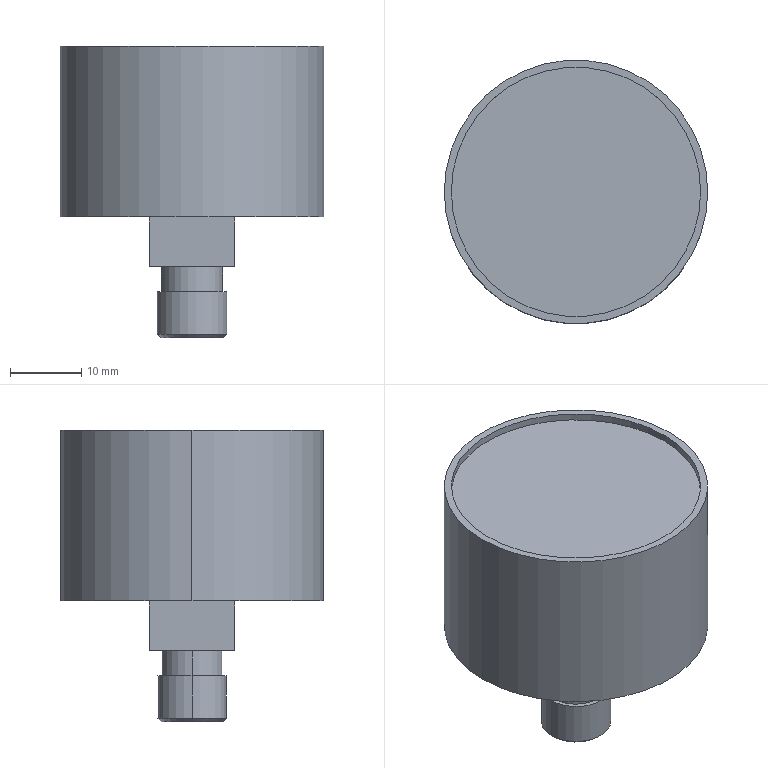Part | NX | 1 solid | 20 faces | box 37 x 37 x 41 mm | volume 26532 mm3 | plane 10 | cylinder 8 | cone 2 | commonest cylinder face diameters 8.57 x2 9.73 x2 35 x2 37 x2
STEP:
#1=CARTESIAN_POINT('',(18.5,0.,0.));
#2=VERTEX_POINT('',#1);
#3=CARTESIAN_POINT('',(-18.5,0.,0.));
#4=VERTEX_POINT('',#3);
#5=CARTESIAN_POINT('',(0.,0.,0.));
#6=DIRECTION('',(0.,0.,-1.));
#7=DIRECTION('',(1.,0.,0.));
#8=AXIS2_PLACEMENT_3D('',#5,#6,#7);
#9=CIRCLE('',#8,18.5);
#10=EDGE_CURVE('',#2,#4,#9,.T.);
#11=ORIENTED_EDGE('',*,*,#10,.T.);
#12=CARTESIAN_POINT('',(-18.5,0.,-24.));
#13=VERTEX_POINT('',#12);
#14=CARTESIAN_POINT('',(-18.5,0.,0.));
#15=DIRECTION('',(0.,0.,1.));
#16=VECTOR('',#15,1000.);
#17=LINE('',#14,#16);
#18=EDGE_CURVE('',#4,#13,#17,.F.);
#19=ORIENTED_EDGE('',*,*,#18,.T.);
#20=CARTESIAN_POINT('',(18.5,0.,-24.));
#21=VERTEX_POINT('',#20);
#22=CARTESIAN_POINT('',(0.,0.,-24.));
#23=DIRECTION('',(0.,0.,1.));
#24=DIRECTION('',(1.,0.,0.));
#25=AXIS2_PLACEMENT_3D('',#22,#23,#24);
#26=CIRCLE('',#25,18.5);
#27=EDGE_CURVE('',#13,#21,#26,.T.);
#28=ORIENTED_EDGE('',*,*,#27,.T.);
#29=CARTESIAN_POINT('',(18.5,0.,0.));
#30=DIRECTION('',(0.,0.,1.));
#31=VECTOR('',#30,1000.);
#32=LINE('',#29,#31);
#33=EDGE_CURVE('',#2,#21,#32,.F.);
#34=ORIENTED_EDGE('',*,*,#33,.F.);
#35=EDGE_LOOP('',(#11,#19,#28,#34));
#36=FACE_BOUND('',#35,.T.);
#37=CARTESIAN_POINT('',(0.,0.,0.));
#38=DIRECTION('',(0.,0.,1.));
#39=DIRECTION('',(1.,0.,0.));
#40=AXIS2_PLACEMENT_3D('',#37,#38,#39);
#41=CYLINDRICAL_SURFACE('',#40,18.5);
#42=ADVANCED_FACE('',(#36),#41,.T.);
#43=CARTESIAN_POINT('',(-4.285,0.,-41.));
#44=VERTEX_POINT('',#43);
#45=CARTESIAN_POINT('',(4.285,0.,-41.));
#46=VERTEX_POINT('',#45);
#47=CARTESIAN_POINT('',(0.,0.,-41.));
#48=DIRECTION('',(0.,0.,1.));
#49=DIRECTION('',(1.,0.,0.));
#50=AXIS2_PLACEMENT_3D('',#47,#48,#49);
#51=CIRCLE('',#50,4.285);
#52=EDGE_CURVE('',#44,#46,#51,.T.);
#53=ORIENTED_EDGE('',*,*,#52,.T.);
#54=CARTESIAN_POINT('',(4.865,0.,-40.5));
#55=VERTEX_POINT('',#54);
#56=CARTESIAN_POINT('',(4.575,0.,-40.75));
#57=DIRECTION('',(0.7574,0.,0.6529));
#58=VECTOR('',#57,1000.);
#59=LINE('',#56,#58);
#60=EDGE_CURVE('',#46,#55,#59,.T.);
#61=ORIENTED_EDGE('',*,*,#60,.T.);
#62=CARTESIAN_POINT('',(-4.865,0.,-40.5));
#63=VERTEX_POINT('',#62);
#64=CARTESIAN_POINT('',(0.,0.,-40.5));
#65=DIRECTION('',(0.,0.,1.));
#66=DIRECTION('',(1.,0.,0.));
#67=AXIS2_PLACEMENT_3D('',#64,#65,#66);
#68=CIRCLE('',#67,4.865);
#69=EDGE_CURVE('',#63,#55,#68,.T.);
#70=ORIENTED_EDGE('',*,*,#69,.F.);
#71=CARTESIAN_POINT('',(-4.575,0.,-40.75));
#72=DIRECTION('',(-0.7574,0.,0.6529));
#73=VECTOR('',#72,1000.);
#74=LINE('',#71,#73);
#75=EDGE_CURVE('',#44,#63,#74,.T.);
#76=ORIENTED_EDGE('',*,*,#75,.F.);
#77=EDGE_LOOP('',(#53,#61,#70,#76));
#78=FACE_BOUND('',#77,.T.);
#79=CARTESIAN_POINT('',(0.,0.,-40.75));
#80=DIRECTION('',(0.,0.,1.));
#81=DIRECTION('',(1.,0.,0.));
#82=AXIS2_PLACEMENT_3D('',#79,#80,#81);
#83=CONICAL_SURFACE('',#82,4.575,0.8593);
#84=ADVANCED_FACE('',(#78),#83,.T.);
#85=ORIENTED_EDGE('',*,*,#10,.F.);
#86=CARTESIAN_POINT('',(0.,0.,0.));
#87=DIRECTION('',(0.,0.,-1.));
#88=DIRECTION('',(1.,0.,0.));
#89=AXIS2_PLACEMENT_3D('',#86,#87,#88);
#90=CIRCLE('',#89,18.5);
#91=EDGE_CURVE('',#4,#2,#90,.T.);
#92=ORIENTED_EDGE('',*,*,#91,.F.);
#93=EDGE_LOOP('',(#85,#92));
#94=FACE_BOUND('',#93,.T.);
#95=CARTESIAN_POINT('',(17.5,0.,0.));
#96=VERTEX_POINT('',#95);
#97=CARTESIAN_POINT('',(-17.5,0.,0.));
#98=VERTEX_POINT('',#97);
#99=CARTESIAN_POINT('',(0.,0.,0.));
#100=DIRECTION('',(0.,0.,1.));
#101=DIRECTION('',(1.,0.,0.));
#102=AXIS2_PLACEMENT_3D('',#99,#100,#101);
#103=CIRCLE('',#102,17.5);
#104=EDGE_CURVE('',#96,#98,#103,.T.);
#105=ORIENTED_EDGE('',*,*,#104,.F.);
#106=CARTESIAN_POINT('',(0.,0.,0.));
#107=DIRECTION('',(0.,0.,1.));
#108=DIRECTION('',(1.,0.,0.));
#109=AXIS2_PLACEMENT_3D('',#106,#107,#108);
#110=CIRCLE('',#109,17.5);
#111=EDGE_CURVE('',#98,#96,#110,.T.);
#112=ORIENTED_EDGE('',*,*,#111,.F.);
#113=EDGE_LOOP('',(#105,#112));
#114=FACE_BOUND('',#113,.T.);
#115=CARTESIAN_POINT('',(0.,0.,0.));
#116=DIRECTION('',(0.,0.,1.));
#117=DIRECTION('',(1.,0.,0.));
#118=AXIS2_PLACEMENT_3D('',#115,#116,#117);
#119=PLANE('',#118);
#120=ADVANCED_FACE('',(#94,#114),#119,.T.);
#121=CARTESIAN_POINT('',(17.5,0.,-1.));
#122=VERTEX_POINT('',#121);
#123=CARTESIAN_POINT('',(-17.5,0.,-1.));
#124=VERTEX_POINT('',#123);
#125=CARTESIAN_POINT('',(0.,0.,-1.));
#126=DIRECTION('',(0.,0.,-1.));
#127=DIRECTION('',(1.,0.,0.));
#128=AXIS2_PLACEMENT_3D('',#125,#126,#127);
#129=CIRCLE('',#128,17.5);
#130=EDGE_CURVE('',#122,#124,#129,.T.);
#131=ORIENTED_EDGE('',*,*,#130,.T.);
#132=CARTESIAN_POINT('',(-17.5,0.,0.));
#133=DIRECTION('',(0.,0.,1.));
#134=VECTOR('',#133,1000.);
#135=LINE('',#132,#134);
#136=EDGE_CURVE('',#98,#124,#135,.F.);
#137=ORIENTED_EDGE('',*,*,#136,.F.);
#138=ORIENTED_EDGE('',*,*,#111,.T.);
#139=CARTESIAN_POINT('',(17.5,0.,0.));
#140=DIRECTION('',(0.,0.,1.));
#141=VECTOR('',#140,1000.);
#142=LINE('',#139,#141);
#143=EDGE_CURVE('',#96,#122,#142,.F.);
#144=ORIENTED_EDGE('',*,*,#143,.T.);
#145=EDGE_LOOP('',(#131,#137,#138,#144));
#146=FACE_BOUND('',#145,.T.);
#147=CARTESIAN_POINT('',(0.,0.,0.));
#148=DIRECTION('',(0.,0.,1.));
#149=DIRECTION('',(1.,0.,0.));
#150=AXIS2_PLACEMENT_3D('',#147,#148,#149);
#151=CYLINDRICAL_SURFACE('',#150,17.5);
#152=ADVANCED_FACE('',(#146),#151,.F.);
#153=ORIENTED_EDGE('',*,*,#52,.F.);
#154=CARTESIAN_POINT('',(0.,0.,-41.));
#155=DIRECTION('',(0.,0.,1.));
#156=DIRECTION('',(1.,0.,0.));
#157=AXIS2_PLACEMENT_3D('',#154,#155,#156);
#158=CIRCLE('',#157,4.285);
#159=EDGE_CURVE('',#46,#44,#158,.T.);
#160=ORIENTED_EDGE('',*,*,#159,.F.);
#161=EDGE_LOOP('',(#153,#160));
#162=FACE_BOUND('',#161,.T.);
#163=CARTESIAN_POINT('',(2.143,0.,-41.));
#164=DIRECTION('',(0.,0.,-1.));
#165=DIRECTION('',(0.,-1.,0.));
#166=AXIS2_PLACEMENT_3D('',#163,#164,#165);
#167=PLANE('',#166);
#168=ADVANCED_FACE('',(#162),#167,.T.);
#169=ORIENTED_EDGE('',*,*,#130,.F.);
#170=CARTESIAN_POINT('',(0.,0.,-1.));
#171=DIRECTION('',(0.,0.,-1.));
#172=DIRECTION('',(1.,0.,0.));
#173=AXIS2_PLACEMENT_3D('',#170,#171,#172);
#174=CIRCLE('',#173,17.5);
#175=EDGE_CURVE('',#124,#122,#174,.T.);
#176=ORIENTED_EDGE('',*,*,#175,.F.);
#177=EDGE_LOOP('',(#169,#176));
#178=FACE_BOUND('',#177,.T.);
#179=CARTESIAN_POINT('',(0.,0.,-1.));
#180=DIRECTION('',(0.,0.,1.));
#181=DIRECTION('',(1.,0.,0.));
#182=AXIS2_PLACEMENT_3D('',#179,#180,#181);
#183=PLANE('',#182);
#184=ADVANCED_FACE('',(#178),#183,.T.);
#185=CARTESIAN_POINT('',(0.,0.,-24.));
#186=DIRECTION('',(0.,0.,1.));
#187=DIRECTION('',(1.,0.,0.));
#188=AXIS2_PLACEMENT_3D('',#185,#186,#187);
#189=CIRCLE('',#188,18.5);
#190=EDGE_CURVE('',#21,#13,#189,.T.);
#191=ORIENTED_EDGE('',*,*,#190,.F.);
#192=ORIENTED_EDGE('',*,*,#27,.F.);
#193=EDGE_LOOP('',(#191,#192));
#194=FACE_BOUND('',#193,.T.);
#195=CARTESIAN_POINT('',(6.,-6.,-24.));
#196=VERTEX_POINT('',#195);
#197=CARTESIAN_POINT('',(6.,6.,-24.));
#198=VERTEX_POINT('',#197);
#199=CARTESIAN_POINT('',(6.,-6.,-24.));
#200=DIRECTION('',(0.,1.,0.));
#201=VECTOR('',#200,1000.);
#202=LINE('',#199,#201);
#203=EDGE_CURVE('',#196,#198,#202,.T.);
#204=ORIENTED_EDGE('',*,*,#203,.T.);
#205=CARTESIAN_POINT('',(-6.,6.,-24.));
#206=VERTEX_POINT('',#205);
#207=CARTESIAN_POINT('',(6.,6.,-24.));
#208=DIRECTION('',(-1.,0.,0.));
#209=VECTOR('',#208,1000.);
#210=LINE('',#207,#209);
#211=EDGE_CURVE('',#198,#206,#210,.T.);
#212=ORIENTED_EDGE('',*,*,#211,.T.);
#213=CARTESIAN_POINT('',(-6.,-6.,-24.));
#214=VERTEX_POINT('',#213);
#215=CARTESIAN_POINT('',(-6.,6.,-24.));
#216=DIRECTION('',(0.,-1.,0.));
#217=VECTOR('',#216,1000.);
#218=LINE('',#215,#217);
#219=EDGE_CURVE('',#206,#214,#218,.T.);
#220=ORIENTED_EDGE('',*,*,#219,.T.);
#221=CARTESIAN_POINT('',(-6.,-6.,-24.));
#222=DIRECTION('',(1.,0.,0.));
#223=VECTOR('',#222,1000.);
#224=LINE('',#221,#223);
#225=EDGE_CURVE('',#214,#196,#224,.T.);
#226=ORIENTED_EDGE('',*,*,#225,.T.);
#227=EDGE_LOOP('',(#204,#212,#220,#226));
#228=FACE_BOUND('',#227,.T.);
#229=CARTESIAN_POINT('',(0.,0.,-24.));
#230=DIRECTION('',(0.,0.,1.));
#231=DIRECTION('',(1.,0.,0.));
#232=AXIS2_PLACEMENT_3D('',#229,#230,#231);
#233=PLANE('',#232);
#234=ADVANCED_FACE('',(#194,#228),#233,.F.);
#235=CARTESIAN_POINT('',(6.,-6.,-31.));
#236=VERTEX_POINT('',#235);
#237=CARTESIAN_POINT('',(6.,6.,-31.));
#238=VERTEX_POINT('',#237);
#239=CARTESIAN_POINT('',(6.,-6.,-31.));
#240=DIRECTION('',(0.,1.,0.));
#241=VECTOR('',#240,1000.);
#242=LINE('',#239,#241);
#243=EDGE_CURVE('',#236,#238,#242,.T.);
#244=ORIENTED_EDGE('',*,*,#243,.T.);
#245=CARTESIAN_POINT('',(6.,6.,-24.));
#246=DIRECTION('',(0.,0.,-1.));
#247=VECTOR('',#246,1000.);
#248=LINE('',#245,#247);
#249=EDGE_CURVE('',#198,#238,#248,.T.);
#250=ORIENTED_EDGE('',*,*,#249,.F.);
#251=ORIENTED_EDGE('',*,*,#203,.F.);
#252=CARTESIAN_POINT('',(6.,-6.,-24.));
#253=DIRECTION('',(0.,0.,-1.));
#254=VECTOR('',#253,1000.);
#255=LINE('',#252,#254);
#256=EDGE_CURVE('',#196,#236,#255,.T.);
#257=ORIENTED_EDGE('',*,*,#256,.T.);
#258=EDGE_LOOP('',(#244,#250,#251,#257));
#259=FACE_BOUND('',#258,.T.);
#260=CARTESIAN_POINT('',(6.,-6.,-24.));
#261=DIRECTION('',(1.,0.,0.));
#262=DIRECTION('',(0.,1.,0.));
#263=AXIS2_PLACEMENT_3D('',#260,#261,#262);
#264=PLANE('',#263);
#265=ADVANCED_FACE('',(#259),#264,.T.);
#266=ORIENTED_EDGE('',*,*,#243,.F.);
#267=CARTESIAN_POINT('',(-6.,-6.,-31.));
#268=VERTEX_POINT('',#267);
#269=CARTESIAN_POINT('',(-6.,-6.,-31.));
#270=DIRECTION('',(1.,0.,0.));
#271=VECTOR('',#270,1000.);
#272=LINE('',#269,#271);
#273=EDGE_CURVE('',#268,#236,#272,.T.);
#274=ORIENTED_EDGE('',*,*,#273,.F.);
#275=CARTESIAN_POINT('',(-6.,6.,-31.));
#276=VERTEX_POINT('',#275);
#277=CARTESIAN_POINT('',(-6.,6.,-31.));
#278=DIRECTION('',(0.,-1.,0.));
#279=VECTOR('',#278,1000.);
#280=LINE('',#277,#279);
#281=EDGE_CURVE('',#276,#268,#280,.T.);
#282=ORIENTED_EDGE('',*,*,#281,.F.);
#283=CARTESIAN_POINT('',(6.,6.,-31.));
#284=DIRECTION('',(-1.,0.,0.));
#285=VECTOR('',#284,1000.);
#286=LINE('',#283,#285);
#287=EDGE_CURVE('',#238,#276,#286,.T.);
#288=ORIENTED_EDGE('',*,*,#287,.F.);
#289=EDGE_LOOP('',(#266,#274,#282,#288));
#290=FACE_BOUND('',#289,.T.);
#291=CARTESIAN_POINT('',(4.285,0.,-31.));
#292=VERTEX_POINT('',#291);
#293=CARTESIAN_POINT('',(-4.285,0.,-31.));
#294=VERTEX_POINT('',#293);
#295=CARTESIAN_POINT('',(0.,0.,-31.));
#296=DIRECTION('',(0.,0.,-1.));
#297=DIRECTION('',(-1.,0.,0.));
#298=AXIS2_PLACEMENT_3D('',#295,#296,#297);
#299=CIRCLE('',#298,4.285);
#300=EDGE_CURVE('',#292,#294,#299,.T.);
#301=ORIENTED_EDGE('',*,*,#300,.F.);
#302=CARTESIAN_POINT('',(0.,0.,-31.));
#303=DIRECTION('',(0.,0.,-1.));
#304=DIRECTION('',(-1.,0.,0.));
#305=AXIS2_PLACEMENT_3D('',#302,#303,#304);
#306=CIRCLE('',#305,4.285);
#307=EDGE_CURVE('',#294,#292,#306,.T.);
#308=ORIENTED_EDGE('',*,*,#307,.F.);
#309=EDGE_LOOP('',(#301,#308));
#310=FACE_BOUND('',#309,.T.);
#311=CARTESIAN_POINT('',(0.,0.,-31.));
#312=DIRECTION('',(0.,0.,1.));
#313=DIRECTION('',(1.,0.,0.));
#314=AXIS2_PLACEMENT_3D('',#311,#312,#313);
#315=PLANE('',#314);
#316=ADVANCED_FACE('',(#290,#310),#315,.F.);
#317=ORIENTED_EDGE('',*,*,#287,.T.);
#318=CARTESIAN_POINT('',(-6.,6.,-24.));
#319=DIRECTION('',(0.,0.,-1.));
#320=VECTOR('',#319,1000.);
#321=LINE('',#318,#320);
#322=EDGE_CURVE('',#206,#276,#321,.T.);
#323=ORIENTED_EDGE('',*,*,#322,.F.);
#324=ORIENTED_EDGE('',*,*,#211,.F.);
#325=ORIENTED_EDGE('',*,*,#249,.T.);
#326=EDGE_LOOP('',(#317,#323,#324,#325));
#327=FACE_BOUND('',#326,.T.);
#328=CARTESIAN_POINT('',(6.,6.,-24.));
#329=DIRECTION('',(0.,1.,0.));
#330=DIRECTION('',(1.,0.,0.));
#331=AXIS2_PLACEMENT_3D('',#328,#329,#330);
#332=PLANE('',#331);
#333=ADVANCED_FACE('',(#327),#332,.T.);
#334=ORIENTED_EDGE('',*,*,#281,.T.);
#335=CARTESIAN_POINT('',(-6.,-6.,-24.));
#336=DIRECTION('',(0.,0.,-1.));
#337=VECTOR('',#336,1000.);
#338=LINE('',#335,#337);
#339=EDGE_CURVE('',#214,#268,#338,.T.);
#340=ORIENTED_EDGE('',*,*,#339,.F.);
#341=ORIENTED_EDGE('',*,*,#219,.F.);
#342=ORIENTED_EDGE('',*,*,#322,.T.);
#343=EDGE_LOOP('',(#334,#340,#341,#342));
#344=FACE_BOUND('',#343,.T.);
#345=CARTESIAN_POINT('',(-6.,6.,-24.));
#346=DIRECTION('',(-1.,0.,0.));
#347=DIRECTION('',(0.,0.,1.));
#348=AXIS2_PLACEMENT_3D('',#345,#346,#347);
#349=PLANE('',#348);
#350=ADVANCED_FACE('',(#344),#349,.T.);
#351=ORIENTED_EDGE('',*,*,#273,.T.);
#352=ORIENTED_EDGE('',*,*,#256,.F.);
#353=ORIENTED_EDGE('',*,*,#225,.F.);
#354=ORIENTED_EDGE('',*,*,#339,.T.);
#355=EDGE_LOOP('',(#351,#352,#353,#354));
#356=FACE_BOUND('',#355,.T.);
#357=CARTESIAN_POINT('',(-6.,-6.,-24.));
#358=DIRECTION('',(0.,-1.,0.));
#359=DIRECTION('',(0.,0.,-1.));
#360=AXIS2_PLACEMENT_3D('',#357,#358,#359);
#361=PLANE('',#360);
#362=ADVANCED_FACE('',(#356),#361,.T.);
#363=CARTESIAN_POINT('',(4.285,0.,-34.49));
#364=VERTEX_POINT('',#363);
#365=CARTESIAN_POINT('',(-4.285,0.,-34.49));
#366=VERTEX_POINT('',#365);
#367=CARTESIAN_POINT('',(0.,0.,-34.49));
#368=DIRECTION('',(0.,0.,1.));
#369=DIRECTION('',(-1.,0.,0.));
#370=AXIS2_PLACEMENT_3D('',#367,#368,#369);
#371=CIRCLE('',#370,4.285);
#372=EDGE_CURVE('',#364,#366,#371,.T.);
#373=ORIENTED_EDGE('',*,*,#372,.T.);
#374=CARTESIAN_POINT('',(-4.285,0.,-32.74));
#375=DIRECTION('',(0.,0.,1.));
#376=VECTOR('',#375,1000.);
#377=LINE('',#374,#376);
#378=EDGE_CURVE('',#294,#366,#377,.F.);
#379=ORIENTED_EDGE('',*,*,#378,.F.);
#380=ORIENTED_EDGE('',*,*,#307,.T.);
#381=CARTESIAN_POINT('',(4.285,0.,-32.74));
#382=DIRECTION('',(0.,0.,1.));
#383=VECTOR('',#382,1000.);
#384=LINE('',#381,#383);
#385=EDGE_CURVE('',#292,#364,#384,.F.);
#386=ORIENTED_EDGE('',*,*,#385,.T.);
#387=EDGE_LOOP('',(#373,#379,#380,#386));
#388=FACE_BOUND('',#387,.T.);
#389=CARTESIAN_POINT('',(0.,0.,-32.74));
#390=DIRECTION('',(0.,0.,1.));
#391=DIRECTION('',(1.,0.,0.));
#392=AXIS2_PLACEMENT_3D('',#389,#390,#391);
#393=CYLINDRICAL_SURFACE('',#392,4.285);
#394=ADVANCED_FACE('',(#388),#393,.T.);
#395=CARTESIAN_POINT('',(4.865,0.,-34.49));
#396=VERTEX_POINT('',#395);
#397=CARTESIAN_POINT('',(-4.865,0.,-34.49));
#398=VERTEX_POINT('',#397);
#399=CARTESIAN_POINT('',(0.,0.,-34.49));
#400=DIRECTION('',(0.,0.,-1.));
#401=DIRECTION('',(-1.,0.,0.));
#402=AXIS2_PLACEMENT_3D('',#399,#400,#401);
#403=CIRCLE('',#402,4.865);
#404=EDGE_CURVE('',#396,#398,#403,.T.);
#405=ORIENTED_EDGE('',*,*,#404,.T.);
#406=CARTESIAN_POINT('',(-4.865,0.,-37.495));
#407=DIRECTION('',(0.,0.,1.));
#408=VECTOR('',#407,1000.);
#409=LINE('',#406,#408);
#410=EDGE_CURVE('',#398,#63,#409,.F.);
#411=ORIENTED_EDGE('',*,*,#410,.T.);
#412=ORIENTED_EDGE('',*,*,#69,.T.);
#413=CARTESIAN_POINT('',(4.865,0.,-37.495));
#414=DIRECTION('',(0.,0.,1.));
#415=VECTOR('',#414,1000.);
#416=LINE('',#413,#415);
#417=EDGE_CURVE('',#396,#55,#416,.F.);
#418=ORIENTED_EDGE('',*,*,#417,.F.);
#419=EDGE_LOOP('',(#405,#411,#412,#418));
#420=FACE_BOUND('',#419,.T.);
#421=CARTESIAN_POINT('',(0.,0.,-37.495));
#422=DIRECTION('',(0.,0.,1.));
#423=DIRECTION('',(1.,0.,0.));
#424=AXIS2_PLACEMENT_3D('',#421,#422,#423);
#425=CYLINDRICAL_SURFACE('',#424,4.865);
#426=ADVANCED_FACE('',(#420),#425,.T.);
#427=ORIENTED_EDGE('',*,*,#404,.F.);
#428=CARTESIAN_POINT('',(0.,0.,-34.49));
#429=DIRECTION('',(0.,0.,-1.));
#430=DIRECTION('',(-1.,0.,0.));
#431=AXIS2_PLACEMENT_3D('',#428,#429,#430);
#432=CIRCLE('',#431,4.865);
#433=EDGE_CURVE('',#398,#396,#432,.T.);
#434=ORIENTED_EDGE('',*,*,#433,.F.);
#435=EDGE_LOOP('',(#427,#434));
#436=FACE_BOUND('',#435,.T.);
#437=ORIENTED_EDGE('',*,*,#372,.F.);
#438=CARTESIAN_POINT('',(0.,0.,-34.49));
#439=DIRECTION('',(0.,0.,1.));
#440=DIRECTION('',(-1.,0.,0.));
#441=AXIS2_PLACEMENT_3D('',#438,#439,#440);
#442=CIRCLE('',#441,4.285);
#443=EDGE_CURVE('',#366,#364,#442,.T.);
#444=ORIENTED_EDGE('',*,*,#443,.F.);
#445=EDGE_LOOP('',(#437,#444));
#446=FACE_BOUND('',#445,.T.);
#447=CARTESIAN_POINT('',(4.575,0.,-34.49));
#448=DIRECTION('',(0.,0.,1.));
#449=DIRECTION('',(1.,0.,0.));
#450=AXIS2_PLACEMENT_3D('',#447,#448,#449);
#451=PLANE('',#450);
#452=ADVANCED_FACE('',(#436,#446),#451,.T.);
#453=CARTESIAN_POINT('',(0.,0.,-40.5));
#454=DIRECTION('',(0.,0.,1.));
#455=DIRECTION('',(1.,0.,0.));
#456=AXIS2_PLACEMENT_3D('',#453,#454,#455);
#457=CIRCLE('',#456,4.865);
#458=EDGE_CURVE('',#55,#63,#457,.T.);
#459=ORIENTED_EDGE('',*,*,#458,.F.);
#460=ORIENTED_EDGE('',*,*,#60,.F.);
#461=ORIENTED_EDGE('',*,*,#159,.T.);
#462=ORIENTED_EDGE('',*,*,#75,.T.);
#463=EDGE_LOOP('',(#459,#460,#461,#462));
#464=FACE_BOUND('',#463,.T.);
#465=CARTESIAN_POINT('',(0.,0.,-40.75));
#466=DIRECTION('',(0.,0.,1.));
#467=DIRECTION('',(1.,0.,0.));
#468=AXIS2_PLACEMENT_3D('',#465,#466,#467);
#469=CONICAL_SURFACE('',#468,4.575,0.8593);
#470=ADVANCED_FACE('',(#464),#469,.T.);
#471=ORIENTED_EDGE('',*,*,#458,.T.);
#472=ORIENTED_EDGE('',*,*,#410,.F.);
#473=ORIENTED_EDGE('',*,*,#433,.T.);
#474=ORIENTED_EDGE('',*,*,#417,.T.);
#475=EDGE_LOOP('',(#471,#472,#473,#474));
#476=FACE_BOUND('',#475,.T.);
#477=CARTESIAN_POINT('',(0.,0.,-37.495));
#478=DIRECTION('',(0.,0.,1.));
#479=DIRECTION('',(1.,0.,0.));
#480=AXIS2_PLACEMENT_3D('',#477,#478,#479);
#481=CYLINDRICAL_SURFACE('',#480,4.865);
#482=ADVANCED_FACE('',(#476),#481,.T.);
#483=ORIENTED_EDGE('',*,*,#104,.T.);
#484=ORIENTED_EDGE('',*,*,#136,.T.);
#485=ORIENTED_EDGE('',*,*,#175,.T.);
#486=ORIENTED_EDGE('',*,*,#143,.F.);
#487=EDGE_LOOP('',(#483,#484,#485,#486));
#488=FACE_BOUND('',#487,.T.);
#489=CARTESIAN_POINT('',(0.,0.,0.));
#490=DIRECTION('',(0.,0.,1.));
#491=DIRECTION('',(1.,0.,0.));
#492=AXIS2_PLACEMENT_3D('',#489,#490,#491);
#493=CYLINDRICAL_SURFACE('',#492,17.5);
#494=ADVANCED_FACE('',(#488),#493,.F.);
#495=ORIENTED_EDGE('',*,*,#300,.T.);
#496=ORIENTED_EDGE('',*,*,#378,.T.);
#497=ORIENTED_EDGE('',*,*,#443,.T.);
#498=ORIENTED_EDGE('',*,*,#385,.F.);
#499=EDGE_LOOP('',(#495,#496,#497,#498));
#500=FACE_BOUND('',#499,.T.);
#501=CARTESIAN_POINT('',(0.,0.,-32.74));
#502=DIRECTION('',(0.,0.,1.));
#503=DIRECTION('',(1.,0.,0.));
#504=AXIS2_PLACEMENT_3D('',#501,#502,#503);
#505=CYLINDRICAL_SURFACE('',#504,4.285);
#506=ADVANCED_FACE('',(#500),#505,.T.);
#507=ORIENTED_EDGE('',*,*,#190,.T.);
#508=ORIENTED_EDGE('',*,*,#18,.F.);
#509=ORIENTED_EDGE('',*,*,#91,.T.);
#510=ORIENTED_EDGE('',*,*,#33,.T.);
#511=EDGE_LOOP('',(#507,#508,#509,#510));
#512=FACE_BOUND('',#511,.T.);
#513=CARTESIAN_POINT('',(0.,0.,0.));
#514=DIRECTION('',(0.,0.,1.));
#515=DIRECTION('',(1.,0.,0.));
#516=AXIS2_PLACEMENT_3D('',#513,#514,#515);
#517=CYLINDRICAL_SURFACE('',#516,18.5);
#518=ADVANCED_FACE('',(#512),#517,.T.);
#519=CLOSED_SHELL('',(#42,#84,#120,#152,#168,#184,#234,#265,#316,#333,#350,#362,#394,#426,#452,#470,#482,#494,#506,#518));
#520=MANIFOLD_SOLID_BREP('',#519);
#521=(LENGTH_UNIT()NAMED_UNIT(*)SI_UNIT(.MILLI.,.METRE.));
#522=UNCERTAINTY_MEASURE_WITH_UNIT(LENGTH_MEASURE(0.00001),#521,'','');
#523=(NAMED_UNIT(*)PLANE_ANGLE_UNIT()SI_UNIT($,.RADIAN.));
#524=(NAMED_UNIT(*)SI_UNIT($,.STERADIAN.)SOLID_ANGLE_UNIT());
#525=(GEOMETRIC_REPRESENTATION_CONTEXT(3)GLOBAL_UNCERTAINTY_ASSIGNED_CONTEXT((#522))GLOBAL_UNIT_ASSIGNED_CONTEXT((#521,#523,#524))REPRESENTATION_CONTEXT('',''));
#526=ADVANCED_BREP_SHAPE_REPRESENTATION('',(#520),#525);